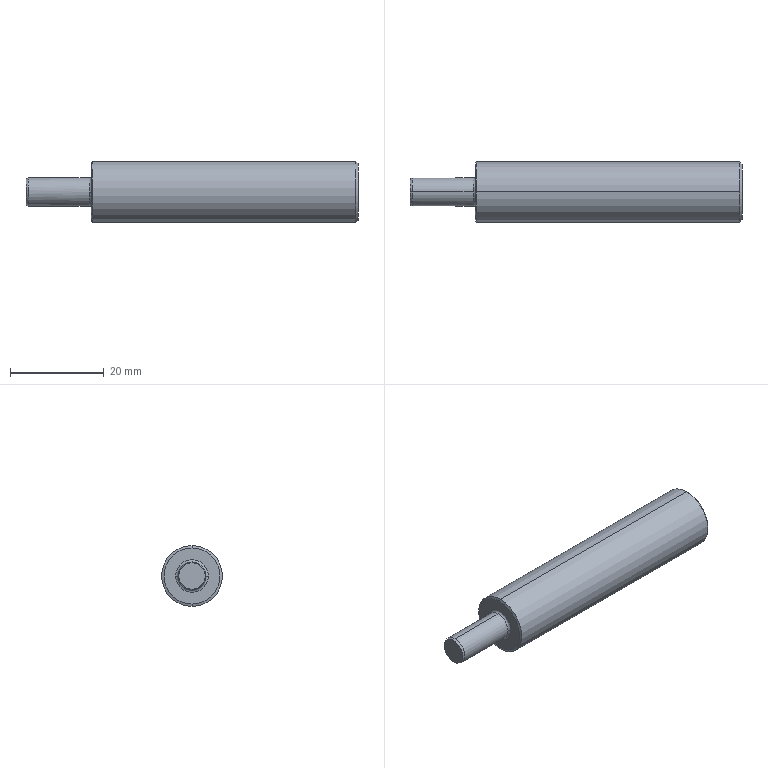Part | STEP file | TQ-DD-AAsfad13_65_f12_b7_p6_n6_2_031010 | 1 solid | 21 faces | box 71 x 13 x 13 mm | volume 7610 mm3 | cone 10 | cylinder 6 | plane 3 | torus 2 | commonest cylinder face diameters 4.917 x2 6 x2 13 x2
STEP:
#1=CARTESIAN_POINT('',(-6.,0.,2.818));
#2=VERTEX_POINT('',#1);
#3=CARTESIAN_POINT('',(-6.,0.,-2.818));
#4=VERTEX_POINT('',#3);
#5=CARTESIAN_POINT('',(-6.,0.,0.));
#6=DIRECTION('',(-1.,0.,0.));
#7=DIRECTION('',(0.,0.,-1.));
#8=AXIS2_PLACEMENT_3D('',#5,#6,#7);
#9=CIRCLE('',#8,2.818);
#10=EDGE_CURVE('',#2,#4,#9,.T.);
#11=ORIENTED_EDGE('',*,*,#10,.F.);
#12=CARTESIAN_POINT('',(-5.5,0.,3.));
#13=VERTEX_POINT('',#12);
#14=CARTESIAN_POINT('',(-6.,0.,2.818));
#15=DIRECTION('',(0.9397,0.,0.342));
#16=VECTOR('',#15,1000.);
#17=LINE('',#14,#16);
#18=EDGE_CURVE('',#2,#13,#17,.T.);
#19=ORIENTED_EDGE('',*,*,#18,.T.);
#20=CARTESIAN_POINT('',(-5.5,0.,-3.));
#21=VERTEX_POINT('',#20);
#22=CARTESIAN_POINT('',(-5.5,0.,0.));
#23=DIRECTION('',(1.,0.,0.));
#24=DIRECTION('',(0.,0.,-1.));
#25=AXIS2_PLACEMENT_3D('',#22,#23,#24);
#26=CIRCLE('',#25,3.);
#27=EDGE_CURVE('',#21,#13,#26,.T.);
#28=ORIENTED_EDGE('',*,*,#27,.F.);
#29=CARTESIAN_POINT('',(-6.,0.,-2.818));
#30=DIRECTION('',(0.9397,0.,-0.342));
#31=VECTOR('',#30,1000.);
#32=LINE('',#29,#31);
#33=EDGE_CURVE('',#4,#21,#32,.T.);
#34=ORIENTED_EDGE('',*,*,#33,.F.);
#35=EDGE_LOOP('',(#11,#19,#28,#34));
#36=FACE_OUTER_BOUND('',#35,.T.);
#37=CARTESIAN_POINT('',(-6.,0.,0.));
#38=DIRECTION('',(1.,0.,0.));
#39=DIRECTION('',(0.,0.,-1.));
#40=AXIS2_PLACEMENT_3D('',#37,#38,#39);
#41=CONICAL_SURFACE('',#40,2.818,0.3491);
#42=ADVANCED_FACE('',(#36),#41,.T.);
#43=CARTESIAN_POINT('',(7.5,3.,0.));
#44=VERTEX_POINT('',#43);
#45=CARTESIAN_POINT('',(7.5,0.,-3.));
#46=VERTEX_POINT('',#45);
#47=CARTESIAN_POINT('',(7.5,0.,0.));
#48=DIRECTION('',(-1.,0.,0.));
#49=DIRECTION('',(0.,-1.,0.));
#50=AXIS2_PLACEMENT_3D('',#47,#48,#49);
#51=CIRCLE('',#50,3.);
#52=EDGE_CURVE('',#44,#46,#51,.T.);
#53=ORIENTED_EDGE('',*,*,#52,.F.);
#54=CARTESIAN_POINT('',(8.,3.5,0.));
#55=VERTEX_POINT('',#54);
#56=CARTESIAN_POINT('',(7.5,3.5,0.));
#57=DIRECTION('',(0.,0.,1.));
#58=DIRECTION('',(0.,-1.,0.));
#59=AXIS2_PLACEMENT_3D('',#56,#57,#58);
#60=CIRCLE('',#59,0.5);
#61=EDGE_CURVE('',#44,#55,#60,.T.);
#62=ORIENTED_EDGE('',*,*,#61,.T.);
#63=CARTESIAN_POINT('',(8.,-3.5,0.));
#64=VERTEX_POINT('',#63);
#65=CARTESIAN_POINT('',(8.,0.,0.));
#66=DIRECTION('',(1.,0.,0.));
#67=DIRECTION('',(0.,-1.,0.));
#68=AXIS2_PLACEMENT_3D('',#65,#66,#67);
#69=CIRCLE('',#68,3.5);
#70=EDGE_CURVE('',#64,#55,#69,.T.);
#71=ORIENTED_EDGE('',*,*,#70,.F.);
#72=CARTESIAN_POINT('',(7.5,-3.,0.));
#73=VERTEX_POINT('',#72);
#74=CARTESIAN_POINT('',(7.5,-3.5,0.));
#75=DIRECTION('',(0.,0.,-1.));
#76=DIRECTION('',(-1.,0.,0.));
#77=AXIS2_PLACEMENT_3D('',#74,#75,#76);
#78=CIRCLE('',#77,0.5);
#79=EDGE_CURVE('',#73,#64,#78,.T.);
#80=ORIENTED_EDGE('',*,*,#79,.F.);
#81=CARTESIAN_POINT('',(7.5,0.,0.));
#82=DIRECTION('',(-1.,0.,0.));
#83=DIRECTION('',(0.,-1.,0.));
#84=AXIS2_PLACEMENT_3D('',#81,#82,#83);
#85=CIRCLE('',#84,3.);
#86=EDGE_CURVE('',#46,#73,#85,.T.);
#87=ORIENTED_EDGE('',*,*,#86,.F.);
#88=EDGE_LOOP('',(#53,#62,#71,#80,#87));
#89=FACE_OUTER_BOUND('',#88,.T.);
#90=CARTESIAN_POINT('',(7.5,0.,0.));
#91=DIRECTION('',(-1.,0.,0.));
#92=DIRECTION('',(0.,-1.,0.));
#93=AXIS2_PLACEMENT_3D('',#90,#91,#92);
#94=TOROIDAL_SURFACE('',#93,3.5,0.5);
#95=ADVANCED_FACE('',(#89),#94,.F.);
#96=CARTESIAN_POINT('',(8.,0.,6.));
#97=VERTEX_POINT('',#96);
#98=CARTESIAN_POINT('',(8.,0.,-6.));
#99=VERTEX_POINT('',#98);
#100=CARTESIAN_POINT('',(8.,0.,0.));
#101=DIRECTION('',(-1.,0.,0.));
#102=DIRECTION('',(0.,-1.,0.));
#103=AXIS2_PLACEMENT_3D('',#100,#101,#102);
#104=CIRCLE('',#103,6.);
#105=EDGE_CURVE('',#97,#99,#104,.T.);
#106=ORIENTED_EDGE('',*,*,#105,.F.);
#107=CARTESIAN_POINT('',(8.182,0.,6.5));
#108=VERTEX_POINT('',#107);
#109=CARTESIAN_POINT('',(8.182,0.,6.5));
#110=DIRECTION('',(0.342,0.,0.9397));
#111=VECTOR('',#110,1000.);
#112=LINE('',#109,#111);
#113=EDGE_CURVE('',#97,#108,#112,.T.);
#114=ORIENTED_EDGE('',*,*,#113,.T.);
#115=CARTESIAN_POINT('',(8.182,0.,-6.5));
#116=VERTEX_POINT('',#115);
#117=CARTESIAN_POINT('',(8.182,0.,0.));
#118=DIRECTION('',(1.,0.,0.));
#119=DIRECTION('',(0.,0.,1.));
#120=AXIS2_PLACEMENT_3D('',#117,#118,#119);
#121=CIRCLE('',#120,6.5);
#122=EDGE_CURVE('',#116,#108,#121,.T.);
#123=ORIENTED_EDGE('',*,*,#122,.F.);
#124=CARTESIAN_POINT('',(8.182,0.,-6.5));
#125=DIRECTION('',(0.342,0.,-0.9397));
#126=VECTOR('',#125,1000.);
#127=LINE('',#124,#126);
#128=EDGE_CURVE('',#99,#116,#127,.T.);
#129=ORIENTED_EDGE('',*,*,#128,.F.);
#130=EDGE_LOOP('',(#106,#114,#123,#129));
#131=FACE_OUTER_BOUND('',#130,.T.);
#132=CARTESIAN_POINT('',(8.182,0.,0.));
#133=DIRECTION('',(1.,0.,0.));
#134=DIRECTION('',(0.,0.,-1.));
#135=AXIS2_PLACEMENT_3D('',#132,#133,#134);
#136=CONICAL_SURFACE('',#135,6.5,1.222);
#137=ADVANCED_FACE('',(#131),#136,.T.);
#138=ORIENTED_EDGE('',*,*,#27,.T.);
#139=CARTESIAN_POINT('',(7.5,0.,3.));
#140=VERTEX_POINT('',#139);
#141=CARTESIAN_POINT('',(-5.9,0.,3.));
#142=DIRECTION('',(1.,0.,0.));
#143=VECTOR('',#142,1000.);
#144=LINE('',#141,#143);
#145=EDGE_CURVE('',#13,#140,#144,.T.);
#146=ORIENTED_EDGE('',*,*,#145,.T.);
#147=CARTESIAN_POINT('',(7.5,0.,0.));
#148=DIRECTION('',(-1.,0.,0.));
#149=DIRECTION('',(0.,-1.,0.));
#150=AXIS2_PLACEMENT_3D('',#147,#148,#149);
#151=CIRCLE('',#150,3.);
#152=EDGE_CURVE('',#140,#44,#151,.T.);
#153=ORIENTED_EDGE('',*,*,#152,.T.);
#154=ORIENTED_EDGE('',*,*,#52,.T.);
#155=CARTESIAN_POINT('',(-5.9,0.,-3.));
#156=DIRECTION('',(1.,0.,0.));
#157=VECTOR('',#156,1000.);
#158=LINE('',#155,#157);
#159=EDGE_CURVE('',#21,#46,#158,.T.);
#160=ORIENTED_EDGE('',*,*,#159,.F.);
#161=EDGE_LOOP('',(#138,#146,#153,#154,#160));
#162=FACE_OUTER_BOUND('',#161,.T.);
#163=CARTESIAN_POINT('',(-5.9,0.,0.));
#164=DIRECTION('',(1.,0.,0.));
#165=DIRECTION('',(0.,0.,-1.));
#166=AXIS2_PLACEMENT_3D('',#163,#164,#165);
#167=CYLINDRICAL_SURFACE('',#166,3.);
#168=ADVANCED_FACE('',(#162),#167,.T.);
#169=CARTESIAN_POINT('',(65.,0.,6.));
#170=VERTEX_POINT('',#169);
#171=CARTESIAN_POINT('',(65.,0.,-6.));
#172=VERTEX_POINT('',#171);
#173=CARTESIAN_POINT('',(65.,0.,0.));
#174=DIRECTION('',(-1.,0.,0.));
#175=DIRECTION('',(0.,0.,1.));
#176=AXIS2_PLACEMENT_3D('',#173,#174,#175);
#177=CIRCLE('',#176,6.);
#178=EDGE_CURVE('',#170,#172,#177,.T.);
#179=ORIENTED_EDGE('',*,*,#178,.T.);
#180=CARTESIAN_POINT('',(64.5,0.,-6.5));
#181=VERTEX_POINT('',#180);
#182=CARTESIAN_POINT('',(64.5,0.,-6.5));
#183=DIRECTION('',(-0.7071,0.,-0.7071));
#184=VECTOR('',#183,1000.);
#185=LINE('',#182,#184);
#186=EDGE_CURVE('',#172,#181,#185,.T.);
#187=ORIENTED_EDGE('',*,*,#186,.T.);
#188=CARTESIAN_POINT('',(64.5,0.,6.5));
#189=VERTEX_POINT('',#188);
#190=CARTESIAN_POINT('',(64.5,0.,0.));
#191=DIRECTION('',(-1.,0.,0.));
#192=DIRECTION('',(0.,0.,-1.));
#193=AXIS2_PLACEMENT_3D('',#190,#191,#192);
#194=CIRCLE('',#193,6.5);
#195=EDGE_CURVE('',#189,#181,#194,.T.);
#196=ORIENTED_EDGE('',*,*,#195,.F.);
#197=CARTESIAN_POINT('',(64.5,0.,6.5));
#198=DIRECTION('',(-0.7071,0.,0.7071));
#199=VECTOR('',#198,1000.);
#200=LINE('',#197,#199);
#201=EDGE_CURVE('',#170,#189,#200,.T.);
#202=ORIENTED_EDGE('',*,*,#201,.F.);
#203=EDGE_LOOP('',(#179,#187,#196,#202));
#204=FACE_OUTER_BOUND('',#203,.T.);
#205=CARTESIAN_POINT('',(64.5,0.,0.));
#206=DIRECTION('',(-1.,0.,0.));
#207=DIRECTION('',(0.,0.,1.));
#208=AXIS2_PLACEMENT_3D('',#205,#206,#207);
#209=CONICAL_SURFACE('',#208,6.5,0.7854);
#210=ADVANCED_FACE('',(#204),#209,.T.);
#211=CARTESIAN_POINT('',(64.459,0.,2.458));
#212=VERTEX_POINT('',#211);
#213=CARTESIAN_POINT('',(64.459,0.,-2.458));
#214=VERTEX_POINT('',#213);
#215=CARTESIAN_POINT('',(64.459,0.,0.));
#216=DIRECTION('',(1.,0.,0.));
#217=DIRECTION('',(0.,1.,0.));
#218=AXIS2_PLACEMENT_3D('',#215,#216,#217);
#219=CIRCLE('',#218,2.458);
#220=EDGE_CURVE('',#212,#214,#219,.T.);
#221=ORIENTED_EDGE('',*,*,#220,.F.);
#222=CARTESIAN_POINT('',(65.,0.,3.));
#223=VERTEX_POINT('',#222);
#224=CARTESIAN_POINT('',(65.,0.,3.));
#225=DIRECTION('',(0.7071,0.,0.7071));
#226=VECTOR('',#225,1000.);
#227=LINE('',#224,#226);
#228=EDGE_CURVE('',#212,#223,#227,.T.);
#229=ORIENTED_EDGE('',*,*,#228,.T.);
#230=CARTESIAN_POINT('',(65.,0.,-3.));
#231=VERTEX_POINT('',#230);
#232=CARTESIAN_POINT('',(65.,0.,0.));
#233=DIRECTION('',(-1.,0.,0.));
#234=DIRECTION('',(0.,0.,-1.));
#235=AXIS2_PLACEMENT_3D('',#232,#233,#234);
#236=CIRCLE('',#235,3.);
#237=EDGE_CURVE('',#231,#223,#236,.T.);
#238=ORIENTED_EDGE('',*,*,#237,.F.);
#239=CARTESIAN_POINT('',(65.,0.,-3.));
#240=DIRECTION('',(0.7071,0.,-0.7071));
#241=VECTOR('',#240,1000.);
#242=LINE('',#239,#241);
#243=EDGE_CURVE('',#214,#231,#242,.T.);
#244=ORIENTED_EDGE('',*,*,#243,.F.);
#245=EDGE_LOOP('',(#221,#229,#238,#244));
#246=FACE_OUTER_BOUND('',#245,.T.);
#247=CARTESIAN_POINT('',(65.,0.,0.));
#248=DIRECTION('',(1.,0.,0.));
#249=DIRECTION('',(0.,0.,-1.));
#250=AXIS2_PLACEMENT_3D('',#247,#248,#249);
#251=CONICAL_SURFACE('',#250,3.,0.7854);
#252=ADVANCED_FACE('',(#246),#251,.F.);
#253=CARTESIAN_POINT('',(47.419,0.,2.459));
#254=VERTEX_POINT('',#253);
#255=CARTESIAN_POINT('',(47.419,0.,-2.459));
#256=VERTEX_POINT('',#255);
#257=CARTESIAN_POINT('',(47.419,0.,0.));
#258=DIRECTION('',(1.,0.,0.));
#259=DIRECTION('',(0.,0.,-1.));
#260=AXIS2_PLACEMENT_3D('',#257,#258,#259);
#261=CIRCLE('',#260,2.458);
#262=EDGE_CURVE('',#254,#256,#261,.T.);
#263=ORIENTED_EDGE('',*,*,#262,.F.);
#264=CARTESIAN_POINT('',(55.939,0.,2.458));
#265=DIRECTION('',(1.,0.,0.));
#266=VECTOR('',#265,1000.);
#267=LINE('',#264,#266);
#268=EDGE_CURVE('',#254,#212,#267,.T.);
#269=ORIENTED_EDGE('',*,*,#268,.T.);
#270=ORIENTED_EDGE('',*,*,#220,.T.);
#271=CARTESIAN_POINT('',(55.939,0.,-2.458));
#272=DIRECTION('',(1.,0.,0.));
#273=VECTOR('',#272,1000.);
#274=LINE('',#271,#273);
#275=EDGE_CURVE('',#256,#214,#274,.T.);
#276=ORIENTED_EDGE('',*,*,#275,.F.);
#277=EDGE_LOOP('',(#263,#269,#270,#276));
#278=FACE_OUTER_BOUND('',#277,.T.);
#279=CARTESIAN_POINT('',(55.939,0.,0.));
#280=DIRECTION('',(1.,0.,0.));
#281=DIRECTION('',(0.,0.,-1.));
#282=AXIS2_PLACEMENT_3D('',#279,#280,#281);
#283=CYLINDRICAL_SURFACE('',#282,2.458);
#284=ADVANCED_FACE('',(#278),#283,.F.);
#285=CARTESIAN_POINT('',(46.,0.,0.));
#286=VERTEX_POINT('',#285);
#287=CARTESIAN_POINT('',(47.419,0.,-2.458));
#288=DIRECTION('',(0.5,0.,-0.866));
#289=VECTOR('',#288,1000.);
#290=LINE('',#287,#289);
#291=EDGE_CURVE('',#286,#256,#290,.T.);
#292=ORIENTED_EDGE('',*,*,#291,.F.);
#293=CARTESIAN_POINT('',(47.419,0.,2.458));
#294=DIRECTION('',(0.5,0.,0.866));
#295=VECTOR('',#294,1000.);
#296=LINE('',#293,#295);
#297=EDGE_CURVE('',#286,#254,#296,.T.);
#298=ORIENTED_EDGE('',*,*,#297,.T.);
#299=ORIENTED_EDGE('',*,*,#262,.T.);
#300=EDGE_LOOP('',(#292,#298,#299));
#301=FACE_OUTER_BOUND('',#300,.T.);
#302=CARTESIAN_POINT('',(47.419,0.,0.));
#303=DIRECTION('',(1.,0.,0.));
#304=DIRECTION('',(0.,0.,-1.));
#305=AXIS2_PLACEMENT_3D('',#302,#303,#304);
#306=CONICAL_SURFACE('',#305,2.458,1.047);
#307=ADVANCED_FACE('',(#301),#306,.F.);
#308=ORIENTED_EDGE('',*,*,#122,.T.);
#309=CARTESIAN_POINT('',(32.5,0.,6.5));
#310=DIRECTION('',(1.,0.,0.));
#311=VECTOR('',#310,1000.);
#312=LINE('',#309,#311);
#313=EDGE_CURVE('',#108,#189,#312,.T.);
#314=ORIENTED_EDGE('',*,*,#313,.T.);
#315=ORIENTED_EDGE('',*,*,#195,.T.);
#316=CARTESIAN_POINT('',(32.5,0.,-6.5));
#317=DIRECTION('',(1.,0.,0.));
#318=VECTOR('',#317,1000.);
#319=LINE('',#316,#318);
#320=EDGE_CURVE('',#116,#181,#319,.T.);
#321=ORIENTED_EDGE('',*,*,#320,.F.);
#322=EDGE_LOOP('',(#308,#314,#315,#321));
#323=FACE_OUTER_BOUND('',#322,.T.);
#324=CARTESIAN_POINT('',(32.5,0.,0.));
#325=DIRECTION('',(1.,0.,0.));
#326=DIRECTION('',(0.,0.,-1.));
#327=AXIS2_PLACEMENT_3D('',#324,#325,#326);
#328=CYLINDRICAL_SURFACE('',#327,6.5);
#329=ADVANCED_FACE('',(#323),#328,.T.);
#330=ORIENTED_EDGE('',*,*,#313,.F.);
#331=CARTESIAN_POINT('',(8.182,0.,0.));
#332=DIRECTION('',(1.,0.,0.));
#333=DIRECTION('',(0.,0.,1.));
#334=AXIS2_PLACEMENT_3D('',#331,#332,#333);
#335=CIRCLE('',#334,6.5);
#336=EDGE_CURVE('',#108,#116,#335,.T.);
#337=ORIENTED_EDGE('',*,*,#336,.T.);
#338=ORIENTED_EDGE('',*,*,#320,.T.);
#339=CARTESIAN_POINT('',(64.5,0.,0.));
#340=DIRECTION('',(-1.,0.,0.));
#341=DIRECTION('',(0.,0.,-1.));
#342=AXIS2_PLACEMENT_3D('',#339,#340,#341);
#343=CIRCLE('',#342,6.5);
#344=EDGE_CURVE('',#181,#189,#343,.T.);
#345=ORIENTED_EDGE('',*,*,#344,.T.);
#346=EDGE_LOOP('',(#330,#337,#338,#345));
#347=FACE_OUTER_BOUND('',#346,.T.);
#348=CARTESIAN_POINT('',(32.5,0.,0.));
#349=DIRECTION('',(1.,0.,0.));
#350=DIRECTION('',(0.,0.,-1.));
#351=AXIS2_PLACEMENT_3D('',#348,#349,#350);
#352=CYLINDRICAL_SURFACE('',#351,6.5);
#353=ADVANCED_FACE('',(#347),#352,.T.);
#354=ORIENTED_EDGE('',*,*,#186,.F.);
#355=CARTESIAN_POINT('',(65.,0.,0.));
#356=DIRECTION('',(-1.,0.,0.));
#357=DIRECTION('',(0.,0.,1.));
#358=AXIS2_PLACEMENT_3D('',#355,#356,#357);
#359=CIRCLE('',#358,6.);
#360=EDGE_CURVE('',#172,#170,#359,.T.);
#361=ORIENTED_EDGE('',*,*,#360,.T.);
#362=ORIENTED_EDGE('',*,*,#201,.T.);
#363=ORIENTED_EDGE('',*,*,#344,.F.);
#364=EDGE_LOOP('',(#354,#361,#362,#363));
#365=FACE_OUTER_BOUND('',#364,.T.);
#366=CARTESIAN_POINT('',(64.5,0.,0.));
#367=DIRECTION('',(-1.,0.,0.));
#368=DIRECTION('',(0.,0.,1.));
#369=AXIS2_PLACEMENT_3D('',#366,#367,#368);
#370=CONICAL_SURFACE('',#369,6.5,0.7854);
#371=ADVANCED_FACE('',(#365),#370,.T.);
#372=ORIENTED_EDGE('',*,*,#178,.F.);
#373=ORIENTED_EDGE('',*,*,#360,.F.);
#374=EDGE_LOOP('',(#372,#373));
#375=FACE_OUTER_BOUND('',#374,.T.);
#376=ORIENTED_EDGE('',*,*,#237,.T.);
#377=CARTESIAN_POINT('',(65.,0.,0.));
#378=DIRECTION('',(-1.,0.,0.));
#379=DIRECTION('',(0.,0.,-1.));
#380=AXIS2_PLACEMENT_3D('',#377,#378,#379);
#381=CIRCLE('',#380,3.);
#382=EDGE_CURVE('',#223,#231,#381,.T.);
#383=ORIENTED_EDGE('',*,*,#382,.T.);
#384=EDGE_LOOP('',(#376,#383));
#385=FACE_BOUND('',#384,.T.);
#386=CARTESIAN_POINT('',(65.,3.,0.));
#387=DIRECTION('',(1.,0.,0.));
#388=DIRECTION('',(0.,0.,-1.));
#389=AXIS2_PLACEMENT_3D('',#386,#387,#388);
#390=PLANE('',#389);
#391=ADVANCED_FACE('',(#375,#385),#390,.T.);
#392=ORIENTED_EDGE('',*,*,#228,.F.);
#393=CARTESIAN_POINT('',(64.459,0.,0.));
#394=DIRECTION('',(1.,0.,0.));
#395=DIRECTION('',(0.,1.,0.));
#396=AXIS2_PLACEMENT_3D('',#393,#394,#395);
#397=CIRCLE('',#396,2.458);
#398=EDGE_CURVE('',#214,#212,#397,.T.);
#399=ORIENTED_EDGE('',*,*,#398,.F.);
#400=ORIENTED_EDGE('',*,*,#243,.T.);
#401=ORIENTED_EDGE('',*,*,#382,.F.);
#402=EDGE_LOOP('',(#392,#399,#400,#401));
#403=FACE_OUTER_BOUND('',#402,.T.);
#404=CARTESIAN_POINT('',(65.,0.,0.));
#405=DIRECTION('',(1.,0.,0.));
#406=DIRECTION('',(0.,0.,-1.));
#407=AXIS2_PLACEMENT_3D('',#404,#405,#406);
#408=CONICAL_SURFACE('',#407,3.,0.7854);
#409=ADVANCED_FACE('',(#403),#408,.F.);
#410=ORIENTED_EDGE('',*,*,#268,.F.);
#411=CARTESIAN_POINT('',(47.419,0.,0.));
#412=DIRECTION('',(1.,0.,0.));
#413=DIRECTION('',(0.,0.,-1.));
#414=AXIS2_PLACEMENT_3D('',#411,#412,#413);
#415=CIRCLE('',#414,2.458);
#416=EDGE_CURVE('',#256,#254,#415,.T.);
#417=ORIENTED_EDGE('',*,*,#416,.F.);
#418=ORIENTED_EDGE('',*,*,#275,.T.);
#419=ORIENTED_EDGE('',*,*,#398,.T.);
#420=EDGE_LOOP('',(#410,#417,#418,#419));
#421=FACE_OUTER_BOUND('',#420,.T.);
#422=CARTESIAN_POINT('',(55.939,0.,0.));
#423=DIRECTION('',(1.,0.,0.));
#424=DIRECTION('',(0.,0.,-1.));
#425=AXIS2_PLACEMENT_3D('',#422,#423,#424);
#426=CYLINDRICAL_SURFACE('',#425,2.458);
#427=ADVANCED_FACE('',(#421),#426,.F.);
#428=ORIENTED_EDGE('',*,*,#297,.F.);
#429=ORIENTED_EDGE('',*,*,#291,.T.);
#430=ORIENTED_EDGE('',*,*,#416,.T.);
#431=EDGE_LOOP('',(#428,#429,#430));
#432=FACE_OUTER_BOUND('',#431,.T.);
#433=CARTESIAN_POINT('',(47.419,0.,0.));
#434=DIRECTION('',(1.,0.,0.));
#435=DIRECTION('',(0.,0.,-1.));
#436=AXIS2_PLACEMENT_3D('',#433,#434,#435);
#437=CONICAL_SURFACE('',#436,2.458,1.047);
#438=ADVANCED_FACE('',(#432),#437,.F.);
#439=ORIENTED_EDGE('',*,*,#70,.T.);
#440=CARTESIAN_POINT('',(8.,0.,0.));
#441=DIRECTION('',(1.,0.,0.));
#442=DIRECTION('',(0.,-1.,0.));
#443=AXIS2_PLACEMENT_3D('',#440,#441,#442);
#444=CIRCLE('',#443,3.5);
#445=EDGE_CURVE('',#55,#64,#444,.T.);
#446=ORIENTED_EDGE('',*,*,#445,.T.);
#447=EDGE_LOOP('',(#439,#446));
#448=FACE_BOUND('',#447,.T.);
#449=CARTESIAN_POINT('',(8.,0.,0.));
#450=DIRECTION('',(-1.,0.,0.));
#451=DIRECTION('',(0.,-1.,0.));
#452=AXIS2_PLACEMENT_3D('',#449,#450,#451);
#453=CIRCLE('',#452,6.);
#454=EDGE_CURVE('',#99,#97,#453,.T.);
#455=ORIENTED_EDGE('',*,*,#454,.T.);
#456=ORIENTED_EDGE('',*,*,#105,.T.);
#457=EDGE_LOOP('',(#455,#456));
#458=FACE_OUTER_BOUND('',#457,.T.);
#459=CARTESIAN_POINT('',(8.,0.,0.));
#460=DIRECTION('',(-1.,0.,0.));
#461=DIRECTION('',(0.,-1.,0.));
#462=AXIS2_PLACEMENT_3D('',#459,#460,#461);
#463=PLANE('',#462);
#464=ADVANCED_FACE('',(#448,#458),#463,.T.);
#465=ORIENTED_EDGE('',*,*,#145,.F.);
#466=CARTESIAN_POINT('',(-5.5,0.,0.));
#467=DIRECTION('',(1.,0.,0.));
#468=DIRECTION('',(0.,0.,-1.));
#469=AXIS2_PLACEMENT_3D('',#466,#467,#468);
#470=CIRCLE('',#469,3.);
#471=EDGE_CURVE('',#13,#21,#470,.T.);
#472=ORIENTED_EDGE('',*,*,#471,.T.);
#473=ORIENTED_EDGE('',*,*,#159,.T.);
#474=ORIENTED_EDGE('',*,*,#86,.T.);
#475=CARTESIAN_POINT('',(7.5,0.,0.));
#476=DIRECTION('',(-1.,0.,0.));
#477=DIRECTION('',(0.,-1.,0.));
#478=AXIS2_PLACEMENT_3D('',#475,#476,#477);
#479=CIRCLE('',#478,3.);
#480=EDGE_CURVE('',#73,#140,#479,.T.);
#481=ORIENTED_EDGE('',*,*,#480,.T.);
#482=EDGE_LOOP('',(#465,#472,#473,#474,#481));
#483=FACE_OUTER_BOUND('',#482,.T.);
#484=CARTESIAN_POINT('',(-5.9,0.,0.));
#485=DIRECTION('',(1.,0.,0.));
#486=DIRECTION('',(0.,0.,-1.));
#487=AXIS2_PLACEMENT_3D('',#484,#485,#486);
#488=CYLINDRICAL_SURFACE('',#487,3.);
#489=ADVANCED_FACE('',(#483),#488,.T.);
#490=ORIENTED_EDGE('',*,*,#113,.F.);
#491=ORIENTED_EDGE('',*,*,#454,.F.);
#492=ORIENTED_EDGE('',*,*,#128,.T.);
#493=ORIENTED_EDGE('',*,*,#336,.F.);
#494=EDGE_LOOP('',(#490,#491,#492,#493));
#495=FACE_OUTER_BOUND('',#494,.T.);
#496=CARTESIAN_POINT('',(8.182,0.,0.));
#497=DIRECTION('',(1.,0.,0.));
#498=DIRECTION('',(0.,0.,-1.));
#499=AXIS2_PLACEMENT_3D('',#496,#497,#498);
#500=CONICAL_SURFACE('',#499,6.5,1.222);
#501=ADVANCED_FACE('',(#495),#500,.T.);
#502=ORIENTED_EDGE('',*,*,#61,.F.);
#503=ORIENTED_EDGE('',*,*,#152,.F.);
#504=ORIENTED_EDGE('',*,*,#480,.F.);
#505=ORIENTED_EDGE('',*,*,#79,.T.);
#506=ORIENTED_EDGE('',*,*,#445,.F.);
#507=EDGE_LOOP('',(#502,#503,#504,#505,#506));
#508=FACE_OUTER_BOUND('',#507,.T.);
#509=CARTESIAN_POINT('',(7.5,0.,0.));
#510=DIRECTION('',(-1.,0.,0.));
#511=DIRECTION('',(0.,-1.,0.));
#512=AXIS2_PLACEMENT_3D('',#509,#510,#511);
#513=TOROIDAL_SURFACE('',#512,3.5,0.5);
#514=ADVANCED_FACE('',(#508),#513,.F.);
#515=CARTESIAN_POINT('',(-6.,0.,0.));
#516=DIRECTION('',(-1.,0.,0.));
#517=DIRECTION('',(0.,0.,-1.));
#518=AXIS2_PLACEMENT_3D('',#515,#516,#517);
#519=CIRCLE('',#518,2.818);
#520=EDGE_CURVE('',#4,#2,#519,.T.);
#521=ORIENTED_EDGE('',*,*,#520,.T.);
#522=ORIENTED_EDGE('',*,*,#10,.T.);
#523=EDGE_LOOP('',(#521,#522));
#524=FACE_OUTER_BOUND('',#523,.T.);
#525=CARTESIAN_POINT('',(-6.,-22.,-7.395));
#526=DIRECTION('',(1.,0.,0.));
#527=DIRECTION('',(0.,0.,-1.));
#528=AXIS2_PLACEMENT_3D('',#525,#526,#527);
#529=PLANE('',#528);
#530=ADVANCED_FACE('',(#524),#529,.F.);
#531=ORIENTED_EDGE('',*,*,#18,.F.);
#532=ORIENTED_EDGE('',*,*,#520,.F.);
#533=ORIENTED_EDGE('',*,*,#33,.T.);
#534=ORIENTED_EDGE('',*,*,#471,.F.);
#535=EDGE_LOOP('',(#531,#532,#533,#534));
#536=FACE_OUTER_BOUND('',#535,.T.);
#537=CARTESIAN_POINT('',(-6.,0.,0.));
#538=DIRECTION('',(1.,0.,0.));
#539=DIRECTION('',(0.,0.,-1.));
#540=AXIS2_PLACEMENT_3D('',#537,#538,#539);
#541=CONICAL_SURFACE('',#540,2.818,0.3491);
#542=ADVANCED_FACE('',(#536),#541,.T.);
#543=CLOSED_SHELL('',(#42,#95,#137,#168,#210,#252,#284,#307,#329,#353,#371,#391,#409,#427,#438,#464,#489,#501,#514,#530,#542));
#544=MANIFOLD_SOLID_BREP('',#543);
#545=CARTESIAN_POINT('',(0.,0.,0.));
#546=DIRECTION('',(0.,0.,1.));
#547=DIRECTION('',(1.,0.,0.));
#548=AXIS2_PLACEMENT_3D('',#545,#546,#547);
#549=(LENGTH_UNIT()NAMED_UNIT(*)SI_UNIT(.MILLI.,.METRE.));
#550=UNCERTAINTY_MEASURE_WITH_UNIT(LENGTH_MEASURE(0.00001),#549,'','');
#551=(NAMED_UNIT(*)PLANE_ANGLE_UNIT()SI_UNIT($,.RADIAN.));
#552=(NAMED_UNIT(*)SI_UNIT($,.STERADIAN.)SOLID_ANGLE_UNIT());
#553=(GEOMETRIC_REPRESENTATION_CONTEXT(3)GLOBAL_UNCERTAINTY_ASSIGNED_CONTEXT((#550))GLOBAL_UNIT_ASSIGNED_CONTEXT((#549,#551,#552))REPRESENTATION_CONTEXT('',''));
#554=ADVANCED_BREP_SHAPE_REPRESENTATION('',(#544,#548),#553);